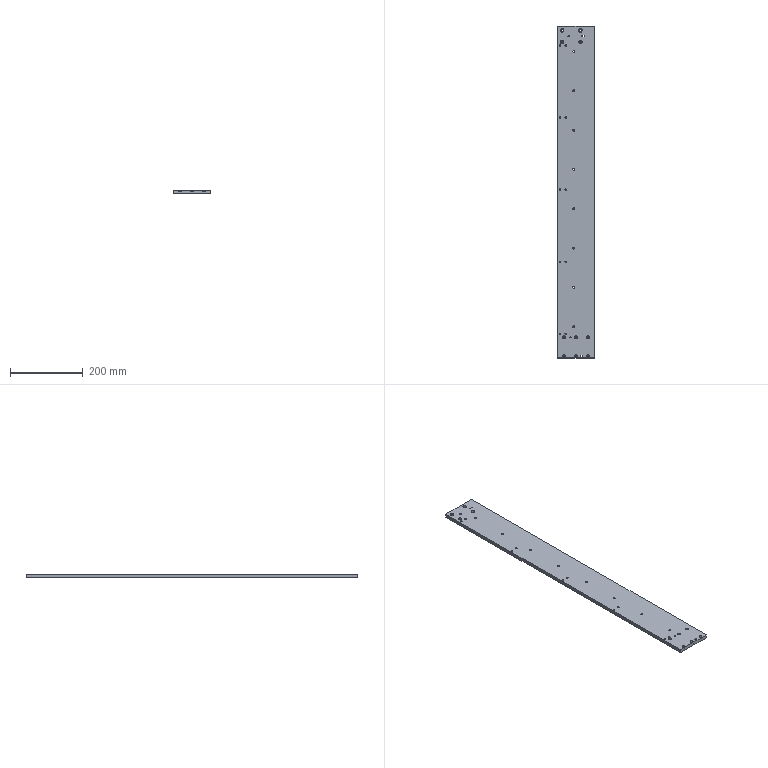Part | STEP file | SynoNew-0304-027 | 1 solid | 100 faces | box 100 x 912 x 10 mm | volume 899646 mm3 | cylinder 62 | plane 38 | commonest cylinder face diameters 4.5 x16 8 x16 5.5 x12 10 x12 3 x3 4 x3